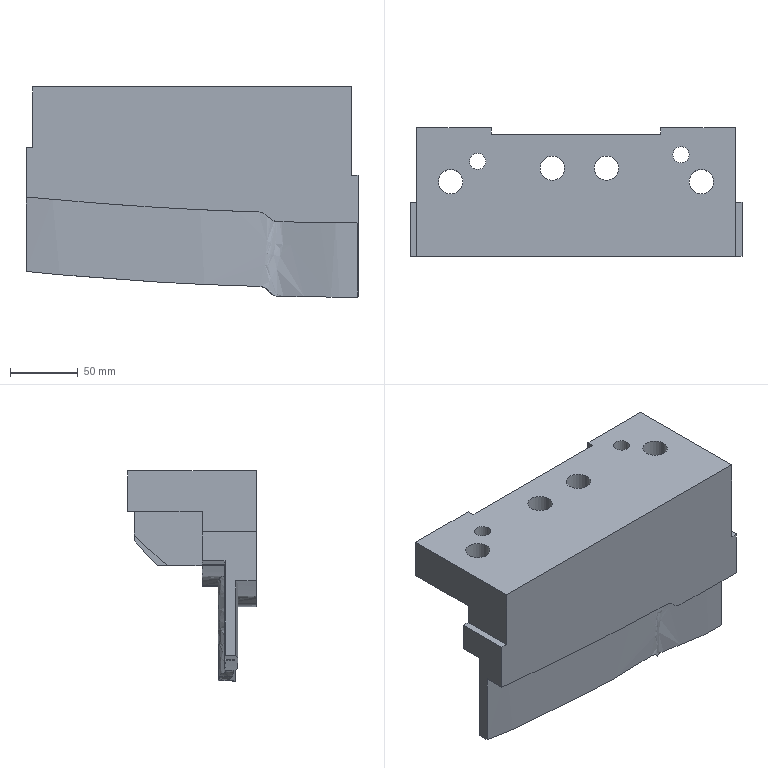Part | NX | features solid 2 | 1 solid | 54 faces | box 245 x 95 x 155.127 mm | volume 1324768 mm3 | plane 31 | spline 12 | cylinder 11 | commonest cylinder face diameters 18 x4 26 x4 12 x2 10 x1